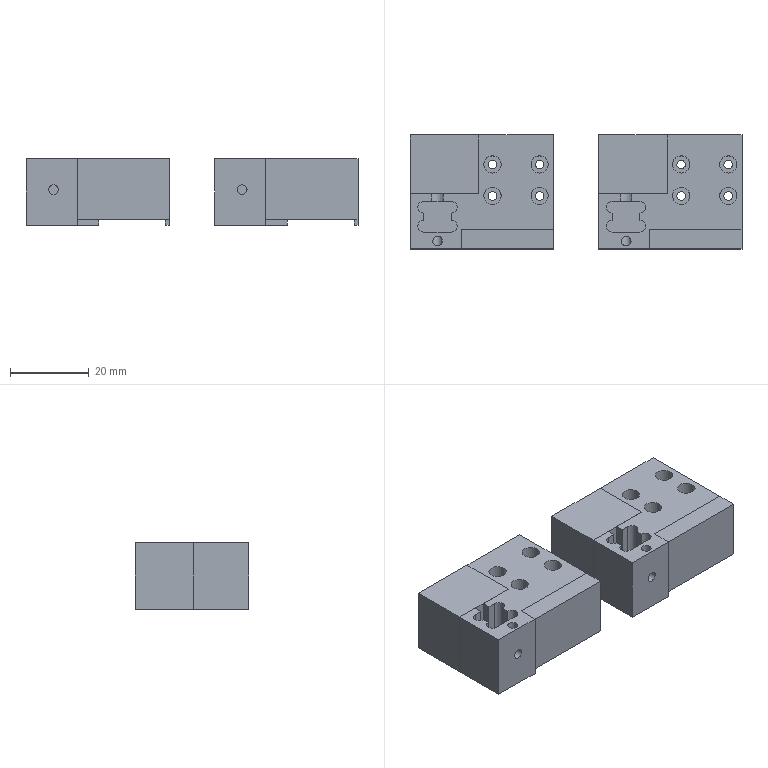NC program | NX | posted with a generic post | part box 84.5 x 29 x 17 mm
Whole program:
N10 G17 G21 G94 G90
(FLOOR_WALL_COPY , TOOL : D63)
N12 T01 M6
N14 G54
N16 G17 G0 G90 X78.75 Y0. B0. C0. S6500 M3
N18 G43 Z30. H1
N20 Z5.
N22 G94 G1 Z2. F1500.
N24 X73.75
N26 X-73.75
N28 X-78.75
N30 Z5.
N32 G0 Z30.
N34 X78.75
N36 Z4.
N38 G1 Z1.
N40 X73.75
N42 X-73.75
N44 X-78.75
N46 Z4.
N48 G0 Z30.
N50 X78.75
N52 Z3.
N54 G1 Z0.
N56 X73.75
N58 X-73.75
N60 X-78.75
N62 Z3.
N64 G0 Z30.
N66 M5
(PLANAR_MILL_COPY , TOOL : D6A45)
N68 T07 M6
N70 G54
N72 G17 G0 G90 X-22.493 Y-1.734 B0. C0. S9500 M3
N74 G43 Z30. H7
N76 Z2.
N78 G94 G1 Z-1. F1250.
N80 G3 X-22.85 Y-2.5 R1.
N82 G1 Y-14.5
N84 G2 X-23.75 Y-15.4 R0.9
N86 G1 X-24.75
N88 G2 X-25.65 Y-14.5 R0.9
N90 G1 Y-0.5
N92 X-42.25
N94 G2 X-43.15 Y0.4 R0.9
N96 G1 Y14.5
N98 G2 X-42.25 Y15.4 R0.9
N100 G1 X-29.25
N102 G2 X-28.35 Y14.5 R0.9
N104 G1 Y10.4
N106 X-23.75
N108 G2 X-22.85 Y9.5 R0.9
N110 G1 Y-2.5
N112 G3 X-22.493 Y-3.266 R1.
N114 G1 Z2.
N116 G0 Z30.
N118 X-8.007
N120 Z2.
N122 G1 Z-1.
N124 G3 X-7.65 Y-2.5 R1.
N126 G1 Y9.5
N128 G2 X-6.75 Y10.4 R0.9
N130 G1 X-5.75
N132 G2 X-4.85 Y9.5 R0.9
N134 G1 Y-14.5
N136 G2 X-5.75 Y-15.4 R0.9
N138 G1 X-6.75
N140 G2 X-7.65 Y-14.5 R0.9
N142 G1 Y-2.5
N144 G3 X-8.007 Y-1.734 R1.
N146 G1 Z2.
N148 G0 Z30.
N150 X25.507
N152 Z2.
N154 G1 Z-1.
N156 G3 X25.15 Y-2.5 R1.
N158 G1 Y-14.5
N160 G2 X24.25 Y-15.4 R0.9
N162 G1 X23.25
N164 G2 X22.35 Y-14.5 R0.9
N166 G1 Y-0.5
N168 X5.75
N170 G2 X4.85 Y0.4 R0.9
N172 G1 Y14.5
N174 G2 X5.75 Y15.4 R0.9
N176 G1 X18.75
N178 G2 X19.65 Y14.5 R0.9
N180 G1 Y10.4
N182 X24.25
N184 G2 X25.15 Y9.5 R0.9
N186 G1 Y-2.5
N188 G3 X25.507 Y-3.266 R1.
N190 G1 Z2.
N192 G0 Z30.
N194 X43.507 Y-1.734
N196 Z2.
N198 G1 Z-1.
N200 G3 X43.15 Y-2.5 R1.
N202 G1 Y-14.5
N204 G2 X42.25 Y-15.4 R0.9
N206 G1 X41.25
N208 G2 X40.35 Y-14.5 R0.9
N210 G1 Y9.5
N212 G2 X41.25 Y10.4 R0.9
N214 G1 X42.25
N216 G2 X43.15 Y9.5 R0.9
N218 G1 Y-2.5
N220 G3 X43.507 Y-3.266 R1.
N222 G1 Z2.
N224 G0 Z30.
N226 M5
N228 M2